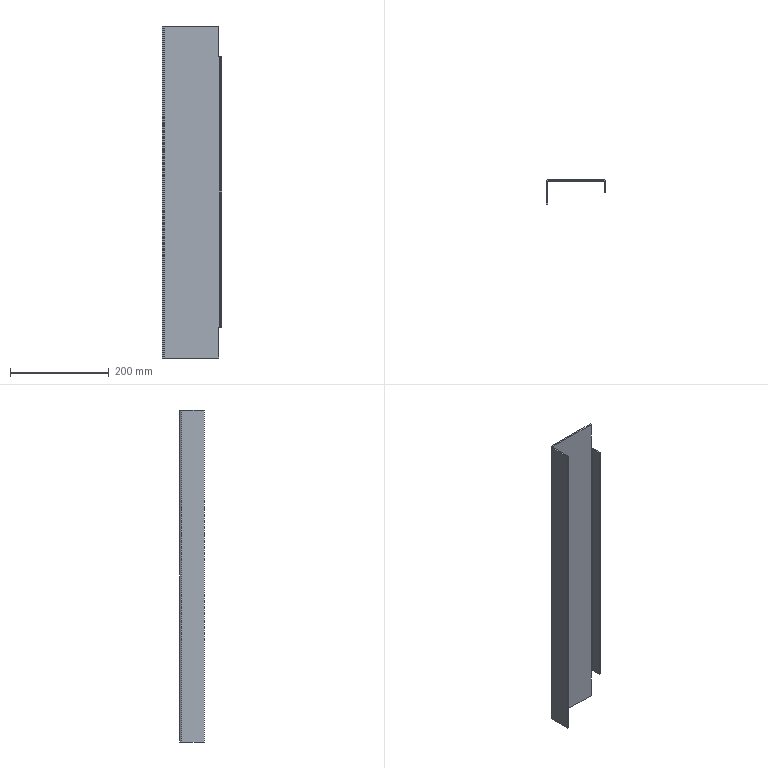Part | STEP file | 中转釜踏Plate 2 | 1 solid | 18 faces | box 120 x 50 x 674 mm | volume 367802 mm3 | plane 14 | cylinder 4 | commonest cylinder face diameters 2 x2 8 x2
STEP:
#1=CARTESIAN_POINT('',(0.,0.,0.));
#2=DIRECTION('',(0.,0.,1.));
#3=DIRECTION('',(1.,0.,0.));
#4=AXIS2_PLACEMENT_3D('',#1,#2,#3);
#5=CARTESIAN_POINT('',(-3.,-25.,275.));
#6=VERTEX_POINT('',#5);
#7=CARTESIAN_POINT('',(-3.,-25.,-275.));
#8=VERTEX_POINT('',#7);
#9=CARTESIAN_POINT('',(-3.,-25.,337.));
#10=DIRECTION('',(0.,0.,-1.));
#11=VECTOR('',#10,1.);
#12=LINE('',#9,#11);
#13=CARTESIAN_POINT('',(-3.,-4.,337.));
#14=DIRECTION('',(1.,0.,0.));
#15=DIRECTION('',(0.,1.,0.));
#16=AXIS2_PLACEMENT_3D('',#13,#14,#15);
#17=PLANE('',#16);
#18=CARTESIAN_POINT('',(-21.,0.));
#19=DIRECTION('',(0.,-1.));
#20=VECTOR('',#19,1.);
#21=LINE('',#18,#20);
#22=(GEOMETRIC_REPRESENTATION_CONTEXT(2)PARAMETRIC_REPRESENTATION_CONTEXT()REPRESENTATION_CONTEXT('',''));
#23=DEFINITIONAL_REPRESENTATION('',(#21),#22);
#24=PCURVE('',#17,#23);
#25=CARTESIAN_POINT('',(0.,-25.,337.));
#26=DIRECTION('',(0.,-1.,0.));
#27=DIRECTION('',(0.,0.,-1.));
#28=AXIS2_PLACEMENT_3D('',#25,#26,#27);
#29=PLANE('',#28);
#30=CARTESIAN_POINT('',(0.,-3.));
#31=DIRECTION('',(1.,0.));
#32=VECTOR('',#31,1.);
#33=LINE('',#30,#32);
#34=(GEOMETRIC_REPRESENTATION_CONTEXT(2)PARAMETRIC_REPRESENTATION_CONTEXT()REPRESENTATION_CONTEXT('',''));
#35=DEFINITIONAL_REPRESENTATION('',(#33),#34);
#36=PCURVE('',#29,#35);
#37=SURFACE_CURVE('',#12,(#24,#36),.PCURVE_S1.);
#38=EDGE_CURVE('',#6,#8,#37,.T.);
#39=ORIENTED_EDGE('',*,*,#38,.F.);
#40=CARTESIAN_POINT('',(-3.,-4.,275.));
#41=VERTEX_POINT('',#40);
#42=CARTESIAN_POINT('',(-3.,-4.,275.));
#43=DIRECTION('',(0.,1.,0.));
#44=VECTOR('',#43,1.);
#45=LINE('',#42,#44);
#46=CARTESIAN_POINT('',(0.,-62.));
#47=DIRECTION('',(1.,0.));
#48=VECTOR('',#47,1.);
#49=LINE('',#46,#48);
#50=(GEOMETRIC_REPRESENTATION_CONTEXT(2)PARAMETRIC_REPRESENTATION_CONTEXT()REPRESENTATION_CONTEXT('',''));
#51=DEFINITIONAL_REPRESENTATION('',(#49),#50);
#52=PCURVE('',#17,#51);
#53=CARTESIAN_POINT('',(0.,-50.,275.));
#54=DIRECTION('',(0.,0.,-1.));
#55=DIRECTION('',(-1.,0.,0.));
#56=AXIS2_PLACEMENT_3D('',#53,#54,#55);
#57=PLANE('',#56);
#58=CARTESIAN_POINT('',(3.,46.));
#59=DIRECTION('',(0.,1.));
#60=VECTOR('',#59,1.);
#61=LINE('',#58,#60);
#62=(GEOMETRIC_REPRESENTATION_CONTEXT(2)PARAMETRIC_REPRESENTATION_CONTEXT()REPRESENTATION_CONTEXT('',''));
#63=DEFINITIONAL_REPRESENTATION('',(#61),#62);
#64=PCURVE('',#57,#63);
#65=SURFACE_CURVE('',#45,(#52,#64),.PCURVE_S1.);
#66=EDGE_CURVE('',#6,#41,#65,.T.);
#67=ORIENTED_EDGE('',*,*,#66,.T.);
#68=CARTESIAN_POINT('',(-3.,-4.,-275.));
#69=VERTEX_POINT('',#68);
#70=CARTESIAN_POINT('',(-3.,-4.,337.));
#71=DIRECTION('',(0.,0.,-1.));
#72=VECTOR('',#71,1.);
#73=LINE('',#70,#72);
#74=CARTESIAN_POINT('',(0.,0.));
#75=DIRECTION('',(0.,-1.));
#76=VECTOR('',#75,1.);
#77=LINE('',#74,#76);
#78=(GEOMETRIC_REPRESENTATION_CONTEXT(2)PARAMETRIC_REPRESENTATION_CONTEXT()REPRESENTATION_CONTEXT('',''));
#79=DEFINITIONAL_REPRESENTATION('',(#77),#78);
#80=PCURVE('',#17,#79);
#81=CARTESIAN_POINT('',(-4.,-4.,337.));
#82=DIRECTION('',(0.,0.,-1.));
#83=DIRECTION('',(-1.,0.,0.));
#84=AXIS2_PLACEMENT_3D('',#81,#82,#83);
#85=CYLINDRICAL_SURFACE('',#84,1.);
#86=CARTESIAN_POINT('',(3.142,0.));
#87=DIRECTION('',(0.,1.));
#88=VECTOR('',#87,1.);
#89=LINE('',#86,#88);
#90=(GEOMETRIC_REPRESENTATION_CONTEXT(2)PARAMETRIC_REPRESENTATION_CONTEXT()REPRESENTATION_CONTEXT('',''));
#91=DEFINITIONAL_REPRESENTATION('',(#89),#90);
#92=PCURVE('',#85,#91);
#93=SURFACE_CURVE('',#73,(#80,#92),.PCURVE_S1.);
#94=EDGE_CURVE('',#41,#69,#93,.T.);
#95=ORIENTED_EDGE('',*,*,#94,.T.);
#96=CARTESIAN_POINT('',(-3.,-4.,-275.));
#97=DIRECTION('',(0.,-1.,0.));
#98=VECTOR('',#97,1.);
#99=LINE('',#96,#98);
#100=CARTESIAN_POINT('',(0.,-612.));
#101=DIRECTION('',(-1.,0.));
#102=VECTOR('',#101,1.);
#103=LINE('',#100,#102);
#104=(GEOMETRIC_REPRESENTATION_CONTEXT(2)PARAMETRIC_REPRESENTATION_CONTEXT()REPRESENTATION_CONTEXT('',''));
#105=DEFINITIONAL_REPRESENTATION('',(#103),#104);
#106=PCURVE('',#17,#105);
#107=CARTESIAN_POINT('',(0.,-50.,-275.));
#108=DIRECTION('',(0.,0.,1.));
#109=DIRECTION('',(1.,0.,0.));
#110=AXIS2_PLACEMENT_3D('',#107,#108,#109);
#111=PLANE('',#110);
#112=CARTESIAN_POINT('',(-3.,46.));
#113=DIRECTION('',(0.,-1.));
#114=VECTOR('',#113,1.);
#115=LINE('',#112,#114);
#116=(GEOMETRIC_REPRESENTATION_CONTEXT(2)PARAMETRIC_REPRESENTATION_CONTEXT()REPRESENTATION_CONTEXT('',''));
#117=DEFINITIONAL_REPRESENTATION('',(#115),#116);
#118=PCURVE('',#111,#117);
#119=SURFACE_CURVE('',#99,(#106,#118),.PCURVE_S1.);
#120=EDGE_CURVE('',#69,#8,#119,.T.);
#121=ORIENTED_EDGE('',*,*,#120,.T.);
#122=EDGE_LOOP('',(#39,#67,#95,#121));
#123=FACE_BOUND('',#122,.T.);
#124=ADVANCED_FACE('',(#123),#17,.F.);
#125=CARTESIAN_POINT('',(0.,-25.,275.));
#126=VERTEX_POINT('',#125);
#127=CARTESIAN_POINT('',(0.,-25.,275.));
#128=DIRECTION('',(1.,0.,0.));
#129=VECTOR('',#128,1.);
#130=LINE('',#127,#129);
#131=CARTESIAN_POINT('',(62.,0.));
#132=DIRECTION('',(0.,1.));
#133=VECTOR('',#132,1.);
#134=LINE('',#131,#133);
#135=(GEOMETRIC_REPRESENTATION_CONTEXT(2)PARAMETRIC_REPRESENTATION_CONTEXT()REPRESENTATION_CONTEXT('',''));
#136=DEFINITIONAL_REPRESENTATION('',(#134),#135);
#137=PCURVE('',#29,#136);
#138=CARTESIAN_POINT('',(0.,25.));
#139=DIRECTION('',(-1.,0.));
#140=VECTOR('',#139,1.);
#141=LINE('',#138,#140);
#142=(GEOMETRIC_REPRESENTATION_CONTEXT(2)PARAMETRIC_REPRESENTATION_CONTEXT()REPRESENTATION_CONTEXT('',''));
#143=DEFINITIONAL_REPRESENTATION('',(#141),#142);
#144=PCURVE('',#57,#143);
#145=SURFACE_CURVE('',#130,(#137,#144),.PCURVE_S1.);
#146=EDGE_CURVE('',#6,#126,#145,.T.);
#147=ORIENTED_EDGE('',*,*,#146,.F.);
#148=ORIENTED_EDGE('',*,*,#38,.T.);
#149=CARTESIAN_POINT('',(0.,-25.,-275.));
#150=VERTEX_POINT('',#149);
#151=CARTESIAN_POINT('',(0.,-25.,-275.));
#152=DIRECTION('',(-1.,0.,0.));
#153=VECTOR('',#152,1.);
#154=LINE('',#151,#153);
#155=CARTESIAN_POINT('',(612.,0.));
#156=DIRECTION('',(0.,-1.));
#157=VECTOR('',#156,1.);
#158=LINE('',#155,#157);
#159=(GEOMETRIC_REPRESENTATION_CONTEXT(2)PARAMETRIC_REPRESENTATION_CONTEXT()REPRESENTATION_CONTEXT('',''));
#160=DEFINITIONAL_REPRESENTATION('',(#158),#159);
#161=PCURVE('',#29,#160);
#162=CARTESIAN_POINT('',(0.,25.));
#163=DIRECTION('',(-1.,0.));
#164=VECTOR('',#163,1.);
#165=LINE('',#162,#164);
#166=(GEOMETRIC_REPRESENTATION_CONTEXT(2)PARAMETRIC_REPRESENTATION_CONTEXT()REPRESENTATION_CONTEXT('',''));
#167=DEFINITIONAL_REPRESENTATION('',(#165),#166);
#168=PCURVE('',#111,#167);
#169=SURFACE_CURVE('',#154,(#161,#168),.PCURVE_S1.);
#170=EDGE_CURVE('',#150,#8,#169,.T.);
#171=ORIENTED_EDGE('',*,*,#170,.F.);
#172=CARTESIAN_POINT('',(0.,-25.,337.));
#173=DIRECTION('',(0.,0.,-1.));
#174=VECTOR('',#173,1.);
#175=LINE('',#172,#174);
#176=CARTESIAN_POINT('',(0.,0.));
#177=DIRECTION('',(1.,0.));
#178=VECTOR('',#177,1.);
#179=LINE('',#176,#178);
#180=(GEOMETRIC_REPRESENTATION_CONTEXT(2)PARAMETRIC_REPRESENTATION_CONTEXT()REPRESENTATION_CONTEXT('',''));
#181=DEFINITIONAL_REPRESENTATION('',(#179),#180);
#182=PCURVE('',#29,#181);
#183=CARTESIAN_POINT('',(0.,-4.,337.));
#184=DIRECTION('',(1.,0.,0.));
#185=DIRECTION('',(0.,1.,0.));
#186=AXIS2_PLACEMENT_3D('',#183,#184,#185);
#187=PLANE('',#186);
#188=CARTESIAN_POINT('',(-21.,0.));
#189=DIRECTION('',(0.,-1.));
#190=VECTOR('',#189,1.);
#191=LINE('',#188,#190);
#192=(GEOMETRIC_REPRESENTATION_CONTEXT(2)PARAMETRIC_REPRESENTATION_CONTEXT()REPRESENTATION_CONTEXT('',''));
#193=DEFINITIONAL_REPRESENTATION('',(#191),#192);
#194=PCURVE('',#187,#193);
#195=SURFACE_CURVE('',#175,(#182,#194),.PCURVE_S1.);
#196=EDGE_CURVE('',#126,#150,#195,.T.);
#197=ORIENTED_EDGE('',*,*,#196,.F.);
#198=EDGE_LOOP('',(#147,#148,#171,#197));
#199=FACE_BOUND('',#198,.T.);
#200=ADVANCED_FACE('',(#199),#29,.T.);
#201=CARTESIAN_POINT('',(0.,-4.,275.));
#202=VERTEX_POINT('',#201);
#203=CARTESIAN_POINT('',(0.,-50.,275.));
#204=DIRECTION('',(0.,1.,0.));
#205=VECTOR('',#204,1.);
#206=LINE('',#203,#205);
#207=CARTESIAN_POINT('',(-46.,-62.));
#208=DIRECTION('',(1.,0.));
#209=VECTOR('',#208,1.);
#210=LINE('',#207,#209);
#211=(GEOMETRIC_REPRESENTATION_CONTEXT(2)PARAMETRIC_REPRESENTATION_CONTEXT()REPRESENTATION_CONTEXT('',''));
#212=DEFINITIONAL_REPRESENTATION('',(#210),#211);
#213=PCURVE('',#187,#212);
#214=CARTESIAN_POINT('',(0.,0.));
#215=DIRECTION('',(0.,1.));
#216=VECTOR('',#215,1.);
#217=LINE('',#214,#216);
#218=(GEOMETRIC_REPRESENTATION_CONTEXT(2)PARAMETRIC_REPRESENTATION_CONTEXT()REPRESENTATION_CONTEXT('',''));
#219=DEFINITIONAL_REPRESENTATION('',(#217),#218);
#220=PCURVE('',#57,#219);
#221=SURFACE_CURVE('',#206,(#213,#220),.PCURVE_S1.);
#222=EDGE_CURVE('',#126,#202,#221,.T.);
#223=ORIENTED_EDGE('',*,*,#222,.F.);
#224=ORIENTED_EDGE('',*,*,#196,.T.);
#225=CARTESIAN_POINT('',(0.,-4.,-275.));
#226=VERTEX_POINT('',#225);
#227=CARTESIAN_POINT('',(0.,-50.,-275.));
#228=DIRECTION('',(0.,1.,0.));
#229=VECTOR('',#228,1.);
#230=LINE('',#227,#229);
#231=CARTESIAN_POINT('',(-46.,-612.));
#232=DIRECTION('',(1.,0.));
#233=VECTOR('',#232,1.);
#234=LINE('',#231,#233);
#235=(GEOMETRIC_REPRESENTATION_CONTEXT(2)PARAMETRIC_REPRESENTATION_CONTEXT()REPRESENTATION_CONTEXT('',''));
#236=DEFINITIONAL_REPRESENTATION('',(#234),#235);
#237=PCURVE('',#187,#236);
#238=CARTESIAN_POINT('',(0.,0.));
#239=DIRECTION('',(0.,1.));
#240=VECTOR('',#239,1.);
#241=LINE('',#238,#240);
#242=(GEOMETRIC_REPRESENTATION_CONTEXT(2)PARAMETRIC_REPRESENTATION_CONTEXT()REPRESENTATION_CONTEXT('',''));
#243=DEFINITIONAL_REPRESENTATION('',(#241),#242);
#244=PCURVE('',#111,#243);
#245=SURFACE_CURVE('',#230,(#237,#244),.PCURVE_S1.);
#246=EDGE_CURVE('',#150,#226,#245,.T.);
#247=ORIENTED_EDGE('',*,*,#246,.T.);
#248=CARTESIAN_POINT('',(0.,-4.,337.));
#249=DIRECTION('',(0.,0.,-1.));
#250=VECTOR('',#249,1.);
#251=LINE('',#248,#250);
#252=CARTESIAN_POINT('',(0.,0.));
#253=DIRECTION('',(0.,-1.));
#254=VECTOR('',#253,1.);
#255=LINE('',#252,#254);
#256=(GEOMETRIC_REPRESENTATION_CONTEXT(2)PARAMETRIC_REPRESENTATION_CONTEXT()REPRESENTATION_CONTEXT('',''));
#257=DEFINITIONAL_REPRESENTATION('',(#255),#256);
#258=PCURVE('',#187,#257);
#259=CARTESIAN_POINT('',(-4.,-4.,337.));
#260=DIRECTION('',(0.,0.,-1.));
#261=DIRECTION('',(-1.,0.,0.));
#262=AXIS2_PLACEMENT_3D('',#259,#260,#261);
#263=CYLINDRICAL_SURFACE('',#262,4.);
#264=CARTESIAN_POINT('',(3.142,0.));
#265=DIRECTION('',(0.,1.));
#266=VECTOR('',#265,1.);
#267=LINE('',#264,#266);
#268=(GEOMETRIC_REPRESENTATION_CONTEXT(2)PARAMETRIC_REPRESENTATION_CONTEXT()REPRESENTATION_CONTEXT('',''));
#269=DEFINITIONAL_REPRESENTATION('',(#267),#268);
#270=PCURVE('',#263,#269);
#271=SURFACE_CURVE('',#251,(#258,#270),.PCURVE_S1.);
#272=EDGE_CURVE('',#202,#226,#271,.T.);
#273=ORIENTED_EDGE('',*,*,#272,.F.);
#274=EDGE_LOOP('',(#223,#224,#247,#273));
#275=FACE_BOUND('',#274,.T.);
#276=ADVANCED_FACE('',(#275),#187,.T.);
#277=CARTESIAN_POINT('',(-4.,0.,275.));
#278=VERTEX_POINT('',#277);
#279=CARTESIAN_POINT('',(-4.,-4.,275.));
#280=DIRECTION('',(0.,0.,1.));
#281=DIRECTION('',(-1.,0.,0.));
#282=AXIS2_PLACEMENT_3D('',#279,#280,#281);
#283=CIRCLE('',#282,4.);
#284=CARTESIAN_POINT('',(6.283,62.));
#285=DIRECTION('',(-1.,0.));
#286=VECTOR('',#285,1.);
#287=LINE('',#284,#286);
#288=(GEOMETRIC_REPRESENTATION_CONTEXT(2)PARAMETRIC_REPRESENTATION_CONTEXT()REPRESENTATION_CONTEXT('',''));
#289=DEFINITIONAL_REPRESENTATION('',(#287),#288);
#290=PCURVE('',#263,#289);
#291=CARTESIAN_POINT('',(8.,46.));
#292=CARTESIAN_POINT('',(8.,39.072));
#293=CARTESIAN_POINT('',(2.,42.536));
#294=CARTESIAN_POINT('',(-4.,46.));
#295=CARTESIAN_POINT('',(2.,49.464));
#296=CARTESIAN_POINT('',(8.,52.928));
#297=CARTESIAN_POINT('',(8.,46.));
#298=(BOUNDED_CURVE()B_SPLINE_CURVE(2,(#291,#292,#293,#294,#295,#296,#297),.UNSPECIFIED.,.T.,.F.)B_SPLINE_CURVE_WITH_KNOTS((1,2,2,2,2,1),(-2.094,0.,2.094,4.189,6.283,8.378),.UNSPECIFIED.)CURVE()GEOMETRIC_REPRESENTATION_ITEM()RATIONAL_B_SPLINE_CURVE((1.,0.5,1.,0.5,1.,0.5,1.))REPRESENTATION_ITEM(''));
#299=(GEOMETRIC_REPRESENTATION_CONTEXT(2)PARAMETRIC_REPRESENTATION_CONTEXT()REPRESENTATION_CONTEXT('',''));
#300=DEFINITIONAL_REPRESENTATION('',(#298),#299);
#301=PCURVE('',#57,#300);
#302=SURFACE_CURVE('',#283,(#290,#301),.PCURVE_S1.);
#303=EDGE_CURVE('',#202,#278,#302,.T.);
#304=ORIENTED_EDGE('',*,*,#303,.F.);
#305=ORIENTED_EDGE('',*,*,#272,.T.);
#306=CARTESIAN_POINT('',(-4.,0.,-275.));
#307=VERTEX_POINT('',#306);
#308=CARTESIAN_POINT('',(-4.,-4.,-275.));
#309=DIRECTION('',(0.,0.,-1.));
#310=DIRECTION('',(1.,0.,0.));
#311=AXIS2_PLACEMENT_3D('',#308,#309,#310);
#312=CIRCLE('',#311,4.);
#313=CARTESIAN_POINT('',(-3.142,612.));
#314=DIRECTION('',(1.,0.));
#315=VECTOR('',#314,1.);
#316=LINE('',#313,#315);
#317=(GEOMETRIC_REPRESENTATION_CONTEXT(2)PARAMETRIC_REPRESENTATION_CONTEXT()REPRESENTATION_CONTEXT('',''));
#318=DEFINITIONAL_REPRESENTATION('',(#316),#317);
#319=PCURVE('',#263,#318);
#320=CARTESIAN_POINT('',(0.,46.));
#321=CARTESIAN_POINT('',(0.,39.072));
#322=CARTESIAN_POINT('',(-6.,42.536));
#323=CARTESIAN_POINT('',(-12.,46.));
#324=CARTESIAN_POINT('',(-6.,49.464));
#325=CARTESIAN_POINT('',(0.,52.928));
#326=CARTESIAN_POINT('',(0.,46.));
#327=(BOUNDED_CURVE()B_SPLINE_CURVE(2,(#320,#321,#322,#323,#324,#325,#326),.UNSPECIFIED.,.T.,.F.)B_SPLINE_CURVE_WITH_KNOTS((1,2,2,2,2,1),(-2.094,0.,2.094,4.189,6.283,8.378),.UNSPECIFIED.)CURVE()GEOMETRIC_REPRESENTATION_ITEM()RATIONAL_B_SPLINE_CURVE((1.,0.5,1.,0.5,1.,0.5,1.))REPRESENTATION_ITEM(''));
#328=(GEOMETRIC_REPRESENTATION_CONTEXT(2)PARAMETRIC_REPRESENTATION_CONTEXT()REPRESENTATION_CONTEXT('',''));
#329=DEFINITIONAL_REPRESENTATION('',(#327),#328);
#330=PCURVE('',#111,#329);
#331=SURFACE_CURVE('',#312,(#319,#330),.PCURVE_S1.);
#332=EDGE_CURVE('',#307,#226,#331,.T.);
#333=ORIENTED_EDGE('',*,*,#332,.F.);
#334=CARTESIAN_POINT('',(-4.,0.,337.));
#335=DIRECTION('',(0.,0.,-1.));
#336=VECTOR('',#335,1.);
#337=LINE('',#334,#336);
#338=CARTESIAN_POINT('',(1.571,0.));
#339=DIRECTION('',(0.,1.));
#340=VECTOR('',#339,1.);
#341=LINE('',#338,#340);
#342=(GEOMETRIC_REPRESENTATION_CONTEXT(2)PARAMETRIC_REPRESENTATION_CONTEXT()REPRESENTATION_CONTEXT('',''));
#343=DEFINITIONAL_REPRESENTATION('',(#341),#342);
#344=PCURVE('',#263,#343);
#345=CARTESIAN_POINT('',(-116.,0.,337.));
#346=DIRECTION('',(0.,1.,0.));
#347=DIRECTION('',(0.,0.,1.));
#348=AXIS2_PLACEMENT_3D('',#345,#346,#347);
#349=PLANE('',#348);
#350=CARTESIAN_POINT('',(0.,112.));
#351=DIRECTION('',(-1.,0.));
#352=VECTOR('',#351,1.);
#353=LINE('',#350,#352);
#354=(GEOMETRIC_REPRESENTATION_CONTEXT(2)PARAMETRIC_REPRESENTATION_CONTEXT()REPRESENTATION_CONTEXT('',''));
#355=DEFINITIONAL_REPRESENTATION('',(#353),#354);
#356=PCURVE('',#349,#355);
#357=SURFACE_CURVE('',#337,(#344,#356),.PCURVE_S1.);
#358=EDGE_CURVE('',#278,#307,#357,.T.);
#359=ORIENTED_EDGE('',*,*,#358,.F.);
#360=EDGE_LOOP('',(#304,#305,#333,#359));
#361=FACE_BOUND('',#360,.T.);
#362=ADVANCED_FACE('',(#361),#263,.T.);
#363=CARTESIAN_POINT('',(-6.,0.,275.));
#364=VERTEX_POINT('',#363);
#365=CARTESIAN_POINT('',(-6.,0.,337.));
#366=VERTEX_POINT('',#365);
#367=CARTESIAN_POINT('',(-6.,0.,337.));
#368=DIRECTION('',(0.,0.,1.));
#369=VECTOR('',#368,1.);
#370=LINE('',#367,#369);
#371=CARTESIAN_POINT('',(0.,110.));
#372=DIRECTION('',(1.,0.));
#373=VECTOR('',#372,1.);
#374=LINE('',#371,#373);
#375=(GEOMETRIC_REPRESENTATION_CONTEXT(2)PARAMETRIC_REPRESENTATION_CONTEXT()REPRESENTATION_CONTEXT('',''));
#376=DEFINITIONAL_REPRESENTATION('',(#374),#375);
#377=PCURVE('',#349,#376);
#378=CARTESIAN_POINT('',(-6.,-50.,337.));
#379=DIRECTION('',(-1.,0.,0.));
#380=DIRECTION('',(0.,0.,1.));
#381=AXIS2_PLACEMENT_3D('',#378,#379,#380);
#382=PLANE('',#381);
#383=CARTESIAN_POINT('',(0.,50.));
#384=DIRECTION('',(1.,0.));
#385=VECTOR('',#384,1.);
#386=LINE('',#383,#385);
#387=(GEOMETRIC_REPRESENTATION_CONTEXT(2)PARAMETRIC_REPRESENTATION_CONTEXT()REPRESENTATION_CONTEXT('',''));
#388=DEFINITIONAL_REPRESENTATION('',(#386),#387);
#389=PCURVE('',#382,#388);
#390=SURFACE_CURVE('',#370,(#377,#389),.PCURVE_S1.);
#391=EDGE_CURVE('',#364,#366,#390,.T.);
#392=ORIENTED_EDGE('',*,*,#391,.F.);
#393=CARTESIAN_POINT('',(-116.,0.,275.));
#394=DIRECTION('',(-1.,0.,0.));
#395=VECTOR('',#394,1.);
#396=LINE('',#393,#395);
#397=CARTESIAN_POINT('',(-62.,0.));
#398=DIRECTION('',(0.,-1.));
#399=VECTOR('',#398,1.);
#400=LINE('',#397,#399);
#401=(GEOMETRIC_REPRESENTATION_CONTEXT(2)PARAMETRIC_REPRESENTATION_CONTEXT()REPRESENTATION_CONTEXT('',''));
#402=DEFINITIONAL_REPRESENTATION('',(#400),#401);
#403=PCURVE('',#349,#402);
#404=CARTESIAN_POINT('',(116.,50.));
#405=DIRECTION('',(1.,0.));
#406=VECTOR('',#405,1.);
#407=LINE('',#404,#406);
#408=(GEOMETRIC_REPRESENTATION_CONTEXT(2)PARAMETRIC_REPRESENTATION_CONTEXT()REPRESENTATION_CONTEXT('',''));
#409=DEFINITIONAL_REPRESENTATION('',(#407),#408);
#410=PCURVE('',#57,#409);
#411=SURFACE_CURVE('',#396,(#403,#410),.PCURVE_S1.);
#412=EDGE_CURVE('',#278,#364,#411,.T.);
#413=ORIENTED_EDGE('',*,*,#412,.F.);
#414=ORIENTED_EDGE('',*,*,#358,.T.);
#415=CARTESIAN_POINT('',(-6.,0.,-275.));
#416=VERTEX_POINT('',#415);
#417=CARTESIAN_POINT('',(-116.,0.,-275.));
#418=DIRECTION('',(1.,0.,0.));
#419=VECTOR('',#418,1.);
#420=LINE('',#417,#419);
#421=CARTESIAN_POINT('',(-612.,0.));
#422=DIRECTION('',(0.,1.));
#423=VECTOR('',#422,1.);
#424=LINE('',#421,#423);
#425=(GEOMETRIC_REPRESENTATION_CONTEXT(2)PARAMETRIC_REPRESENTATION_CONTEXT()REPRESENTATION_CONTEXT('',''));
#426=DEFINITIONAL_REPRESENTATION('',(#424),#425);
#427=PCURVE('',#349,#426);
#428=CARTESIAN_POINT('',(-116.,50.));
#429=DIRECTION('',(1.,0.));
#430=VECTOR('',#429,1.);
#431=LINE('',#428,#430);
#432=(GEOMETRIC_REPRESENTATION_CONTEXT(2)PARAMETRIC_REPRESENTATION_CONTEXT()REPRESENTATION_CONTEXT('',''));
#433=DEFINITIONAL_REPRESENTATION('',(#431),#432);
#434=PCURVE('',#111,#433);
#435=SURFACE_CURVE('',#420,(#427,#434),.PCURVE_S1.);
#436=EDGE_CURVE('',#416,#307,#435,.T.);
#437=ORIENTED_EDGE('',*,*,#436,.F.);
#438=CARTESIAN_POINT('',(-6.,0.,-337.));
#439=VERTEX_POINT('',#438);
#440=CARTESIAN_POINT('',(-6.,0.,337.));
#441=DIRECTION('',(0.,0.,1.));
#442=VECTOR('',#441,1.);
#443=LINE('',#440,#442);
#444=CARTESIAN_POINT('',(0.,110.));
#445=DIRECTION('',(1.,0.));
#446=VECTOR('',#445,1.);
#447=LINE('',#444,#446);
#448=(GEOMETRIC_REPRESENTATION_CONTEXT(2)PARAMETRIC_REPRESENTATION_CONTEXT()REPRESENTATION_CONTEXT('',''));
#449=DEFINITIONAL_REPRESENTATION('',(#447),#448);
#450=PCURVE('',#349,#449);
#451=CARTESIAN_POINT('',(-6.,-50.,-337.));
#452=DIRECTION('',(-1.,0.,0.));
#453=DIRECTION('',(0.,0.,1.));
#454=AXIS2_PLACEMENT_3D('',#451,#452,#453);
#455=PLANE('',#454);
#456=CARTESIAN_POINT('',(674.,50.));
#457=DIRECTION('',(1.,0.));
#458=VECTOR('',#457,1.);
#459=LINE('',#456,#458);
#460=(GEOMETRIC_REPRESENTATION_CONTEXT(2)PARAMETRIC_REPRESENTATION_CONTEXT()REPRESENTATION_CONTEXT('',''));
#461=DEFINITIONAL_REPRESENTATION('',(#459),#460);
#462=PCURVE('',#455,#461);
#463=SURFACE_CURVE('',#443,(#450,#462),.PCURVE_S1.);
#464=EDGE_CURVE('',#439,#416,#463,.T.);
#465=ORIENTED_EDGE('',*,*,#464,.F.);
#466=CARTESIAN_POINT('',(-116.,0.,-337.));
#467=VERTEX_POINT('',#466);
#468=CARTESIAN_POINT('',(-116.,0.,-337.));
#469=DIRECTION('',(1.,0.,0.));
#470=VECTOR('',#469,1.);
#471=LINE('',#468,#470);
#472=CARTESIAN_POINT('',(-674.,0.));
#473=DIRECTION('',(0.,1.));
#474=VECTOR('',#473,1.);
#475=LINE('',#472,#474);
#476=(GEOMETRIC_REPRESENTATION_CONTEXT(2)PARAMETRIC_REPRESENTATION_CONTEXT()REPRESENTATION_CONTEXT('',''));
#477=DEFINITIONAL_REPRESENTATION('',(#475),#476);
#478=PCURVE('',#349,#477);
#479=CARTESIAN_POINT('',(-4.,-4.,-337.));
#480=DIRECTION('',(0.,0.,-1.));
#481=DIRECTION('',(-1.,0.,0.));
#482=AXIS2_PLACEMENT_3D('',#479,#480,#481);
#483=PLANE('',#482);
#484=CARTESIAN_POINT('',(112.,4.));
#485=DIRECTION('',(-1.,0.));
#486=VECTOR('',#485,1.);
#487=LINE('',#484,#486);
#488=(GEOMETRIC_REPRESENTATION_CONTEXT(2)PARAMETRIC_REPRESENTATION_CONTEXT()REPRESENTATION_CONTEXT('',''));
#489=DEFINITIONAL_REPRESENTATION('',(#487),#488);
#490=PCURVE('',#483,#489);
#491=SURFACE_CURVE('',#471,(#478,#490),.PCURVE_S1.);
#492=EDGE_CURVE('',#467,#439,#491,.T.);
#493=ORIENTED_EDGE('',*,*,#492,.F.);
#494=CARTESIAN_POINT('',(-116.,0.,337.));
#495=VERTEX_POINT('',#494);
#496=CARTESIAN_POINT('',(-116.,0.,337.));
#497=DIRECTION('',(0.,0.,-1.));
#498=VECTOR('',#497,1.);
#499=LINE('',#496,#498);
#500=CARTESIAN_POINT('',(0.,0.));
#501=DIRECTION('',(-1.,0.));
#502=VECTOR('',#501,1.);
#503=LINE('',#500,#502);
#504=(GEOMETRIC_REPRESENTATION_CONTEXT(2)PARAMETRIC_REPRESENTATION_CONTEXT()REPRESENTATION_CONTEXT('',''));
#505=DEFINITIONAL_REPRESENTATION('',(#503),#504);
#506=PCURVE('',#349,#505);
#507=CARTESIAN_POINT('',(-116.,-4.,337.));
#508=DIRECTION('',(0.,0.,-1.));
#509=DIRECTION('',(-1.,0.,0.));
#510=AXIS2_PLACEMENT_3D('',#507,#508,#509);
#511=CYLINDRICAL_SURFACE('',#510,4.);
#512=CARTESIAN_POINT('',(1.571,0.));
#513=DIRECTION('',(0.,1.));
#514=VECTOR('',#513,1.);
#515=LINE('',#512,#514);
#516=(GEOMETRIC_REPRESENTATION_CONTEXT(2)PARAMETRIC_REPRESENTATION_CONTEXT()REPRESENTATION_CONTEXT('',''));
#517=DEFINITIONAL_REPRESENTATION('',(#515),#516);
#518=PCURVE('',#511,#517);
#519=SURFACE_CURVE('',#499,(#506,#518),.PCURVE_S1.);
#520=EDGE_CURVE('',#495,#467,#519,.T.);
#521=ORIENTED_EDGE('',*,*,#520,.F.);
#522=CARTESIAN_POINT('',(-116.,0.,337.));
#523=DIRECTION('',(1.,0.,0.));
#524=VECTOR('',#523,1.);
#525=LINE('',#522,#524);
#526=CARTESIAN_POINT('',(0.,0.));
#527=DIRECTION('',(0.,1.));
#528=VECTOR('',#527,1.);
#529=LINE('',#526,#528);
#530=(GEOMETRIC_REPRESENTATION_CONTEXT(2)PARAMETRIC_REPRESENTATION_CONTEXT()REPRESENTATION_CONTEXT('',''));
#531=DEFINITIONAL_REPRESENTATION('',(#529),#530);
#532=PCURVE('',#349,#531);
#533=CARTESIAN_POINT('',(-4.,-4.,337.));
#534=DIRECTION('',(0.,0.,-1.));
#535=DIRECTION('',(-1.,0.,0.));
#536=AXIS2_PLACEMENT_3D('',#533,#534,#535);
#537=PLANE('',#536);
#538=CARTESIAN_POINT('',(112.,4.));
#539=DIRECTION('',(-1.,0.));
#540=VECTOR('',#539,1.);
#541=LINE('',#538,#540);
#542=(GEOMETRIC_REPRESENTATION_CONTEXT(2)PARAMETRIC_REPRESENTATION_CONTEXT()REPRESENTATION_CONTEXT('',''));
#543=DEFINITIONAL_REPRESENTATION('',(#541),#542);
#544=PCURVE('',#537,#543);
#545=SURFACE_CURVE('',#525,(#532,#544),.PCURVE_S1.);
#546=EDGE_CURVE('',#495,#366,#545,.T.);
#547=ORIENTED_EDGE('',*,*,#546,.T.);
#548=EDGE_LOOP('',(#392,#413,#414,#437,#465,#493,#521,#547));
#549=FACE_BOUND('',#548,.T.);
#550=ADVANCED_FACE('',(#549),#349,.T.);
#551=CARTESIAN_POINT('',(-120.,-4.,-337.));
#552=VERTEX_POINT('',#551);
#553=CARTESIAN_POINT('',(-116.,-4.,-337.));
#554=DIRECTION('',(0.,0.,-1.));
#555=DIRECTION('',(1.,0.,0.));
#556=AXIS2_PLACEMENT_3D('',#553,#554,#555);
#557=CIRCLE('',#556,4.);
#558=CARTESIAN_POINT('',(-3.142,674.));
#559=DIRECTION('',(1.,0.));
#560=VECTOR('',#559,1.);
#561=LINE('',#558,#560);
#562=(GEOMETRIC_REPRESENTATION_CONTEXT(2)PARAMETRIC_REPRESENTATION_CONTEXT()REPRESENTATION_CONTEXT('',''));
#563=DEFINITIONAL_REPRESENTATION('',(#561),#562);
#564=PCURVE('',#511,#563);
#565=CARTESIAN_POINT('',(112.,0.));
#566=DIRECTION('',(-1.,0.));
#567=AXIS2_PLACEMENT_2D('',#565,#566);
#568=CIRCLE('',#567,4.);
#569=(GEOMETRIC_REPRESENTATION_CONTEXT(2)PARAMETRIC_REPRESENTATION_CONTEXT()REPRESENTATION_CONTEXT('',''));
#570=DEFINITIONAL_REPRESENTATION('',(#568),#569);
#571=PCURVE('',#483,#570);
#572=SURFACE_CURVE('',#557,(#564,#571),.PCURVE_S1.);
#573=EDGE_CURVE('',#552,#467,#572,.T.);
#574=ORIENTED_EDGE('',*,*,#573,.F.);
#575=CARTESIAN_POINT('',(-120.,-4.,337.));
#576=VERTEX_POINT('',#575);
#577=CARTESIAN_POINT('',(-120.,-4.,337.));
#578=DIRECTION('',(0.,0.,-1.));
#579=VECTOR('',#578,1.);
#580=LINE('',#577,#579);
#581=CARTESIAN_POINT('',(0.,0.));
#582=DIRECTION('',(0.,1.));
#583=VECTOR('',#582,1.);
#584=LINE('',#581,#583);
#585=(GEOMETRIC_REPRESENTATION_CONTEXT(2)PARAMETRIC_REPRESENTATION_CONTEXT()REPRESENTATION_CONTEXT('',''));
#586=DEFINITIONAL_REPRESENTATION('',(#584),#585);
#587=PCURVE('',#511,#586);
#588=CARTESIAN_POINT('',(-120.,-4.,337.));
#589=DIRECTION('',(-1.,0.,0.));
#590=DIRECTION('',(0.,0.,1.));
#591=AXIS2_PLACEMENT_3D('',#588,#589,#590);
#592=PLANE('',#591);
#593=CARTESIAN_POINT('',(0.,0.));
#594=DIRECTION('',(-1.,0.));
#595=VECTOR('',#594,1.);
#596=LINE('',#593,#595);
#597=(GEOMETRIC_REPRESENTATION_CONTEXT(2)PARAMETRIC_REPRESENTATION_CONTEXT()REPRESENTATION_CONTEXT('',''));
#598=DEFINITIONAL_REPRESENTATION('',(#596),#597);
#599=PCURVE('',#592,#598);
#600=SURFACE_CURVE('',#580,(#587,#599),.PCURVE_S1.);
#601=EDGE_CURVE('',#576,#552,#600,.T.);
#602=ORIENTED_EDGE('',*,*,#601,.F.);
#603=CARTESIAN_POINT('',(-116.,-4.,337.));
#604=DIRECTION('',(0.,0.,-1.));
#605=DIRECTION('',(1.,0.,0.));
#606=AXIS2_PLACEMENT_3D('',#603,#604,#605);
#607=CIRCLE('',#606,4.);
#608=CARTESIAN_POINT('',(-3.142,0.));
#609=DIRECTION('',(1.,0.));
#610=VECTOR('',#609,1.);
#611=LINE('',#608,#610);
#612=(GEOMETRIC_REPRESENTATION_CONTEXT(2)PARAMETRIC_REPRESENTATION_CONTEXT()REPRESENTATION_CONTEXT('',''));
#613=DEFINITIONAL_REPRESENTATION('',(#611),#612);
#614=PCURVE('',#511,#613);
#615=CARTESIAN_POINT('',(112.,0.));
#616=DIRECTION('',(-1.,0.));
#617=AXIS2_PLACEMENT_2D('',#615,#616);
#618=CIRCLE('',#617,4.);
#619=(GEOMETRIC_REPRESENTATION_CONTEXT(2)PARAMETRIC_REPRESENTATION_CONTEXT()REPRESENTATION_CONTEXT('',''));
#620=DEFINITIONAL_REPRESENTATION('',(#618),#619);
#621=PCURVE('',#537,#620);
#622=SURFACE_CURVE('',#607,(#614,#621),.PCURVE_S1.);
#623=EDGE_CURVE('',#576,#495,#622,.T.);
#624=ORIENTED_EDGE('',*,*,#623,.T.);
#625=ORIENTED_EDGE('',*,*,#520,.T.);
#626=EDGE_LOOP('',(#574,#602,#624,#625));
#627=FACE_BOUND('',#626,.T.);
#628=ADVANCED_FACE('',(#627),#511,.T.);
#629=CARTESIAN_POINT('',(-120.,-50.,-337.));
#630=VERTEX_POINT('',#629);
#631=CARTESIAN_POINT('',(-120.,-4.,-337.));
#632=DIRECTION('',(0.,1.,0.));
#633=VECTOR('',#632,1.);
#634=LINE('',#631,#633);
#635=CARTESIAN_POINT('',(-674.,0.));
#636=DIRECTION('',(0.,1.));
#637=VECTOR('',#636,1.);
#638=LINE('',#635,#637);
#639=(GEOMETRIC_REPRESENTATION_CONTEXT(2)PARAMETRIC_REPRESENTATION_CONTEXT()REPRESENTATION_CONTEXT('',''));
#640=DEFINITIONAL_REPRESENTATION('',(#638),#639);
#641=PCURVE('',#592,#640);
#642=CARTESIAN_POINT('',(116.,0.));
#643=DIRECTION('',(0.,1.));
#644=VECTOR('',#643,1.);
#645=LINE('',#642,#644);
#646=(GEOMETRIC_REPRESENTATION_CONTEXT(2)PARAMETRIC_REPRESENTATION_CONTEXT()REPRESENTATION_CONTEXT('',''));
#647=DEFINITIONAL_REPRESENTATION('',(#645),#646);
#648=PCURVE('',#483,#647);
#649=SURFACE_CURVE('',#634,(#641,#648),.PCURVE_S1.);
#650=EDGE_CURVE('',#630,#552,#649,.T.);
#651=ORIENTED_EDGE('',*,*,#650,.F.);
#652=CARTESIAN_POINT('',(-120.,-50.,337.));
#653=VERTEX_POINT('',#652);
#654=CARTESIAN_POINT('',(-120.,-50.,337.));
#655=DIRECTION('',(0.,0.,-1.));
#656=VECTOR('',#655,1.);
#657=LINE('',#654,#656);
#658=CARTESIAN_POINT('',(0.,-46.));
#659=DIRECTION('',(-1.,0.));
#660=VECTOR('',#659,1.);
#661=LINE('',#658,#660);
#662=(GEOMETRIC_REPRESENTATION_CONTEXT(2)PARAMETRIC_REPRESENTATION_CONTEXT()REPRESENTATION_CONTEXT('',''));
#663=DEFINITIONAL_REPRESENTATION('',(#661),#662);
#664=PCURVE('',#592,#663);
#665=CARTESIAN_POINT('',(-117.,-50.,337.));
#666=DIRECTION('',(0.,-1.,0.));
#667=DIRECTION('',(0.,0.,-1.));
#668=AXIS2_PLACEMENT_3D('',#665,#666,#667);
#669=PLANE('',#668);
#670=CARTESIAN_POINT('',(0.,-3.));
#671=DIRECTION('',(1.,0.));
#672=VECTOR('',#671,1.);
#673=LINE('',#670,#672);
#674=(GEOMETRIC_REPRESENTATION_CONTEXT(2)PARAMETRIC_REPRESENTATION_CONTEXT()REPRESENTATION_CONTEXT('',''));
#675=DEFINITIONAL_REPRESENTATION('',(#673),#674);
#676=PCURVE('',#669,#675);
#677=SURFACE_CURVE('',#657,(#664,#676),.PCURVE_S1.);
#678=EDGE_CURVE('',#653,#630,#677,.T.);
#679=ORIENTED_EDGE('',*,*,#678,.F.);
#680=CARTESIAN_POINT('',(-120.,-4.,337.));
#681=DIRECTION('',(0.,1.,0.));
#682=VECTOR('',#681,1.);
#683=LINE('',#680,#682);
#684=CARTESIAN_POINT('',(0.,0.));
#685=DIRECTION('',(0.,1.));
#686=VECTOR('',#685,1.);
#687=LINE('',#684,#686);
#688=(GEOMETRIC_REPRESENTATION_CONTEXT(2)PARAMETRIC_REPRESENTATION_CONTEXT()REPRESENTATION_CONTEXT('',''));
#689=DEFINITIONAL_REPRESENTATION('',(#687),#688);
#690=PCURVE('',#592,#689);
#691=CARTESIAN_POINT('',(116.,0.));
#692=DIRECTION('',(0.,1.));
#693=VECTOR('',#692,1.);
#694=LINE('',#691,#693);
#695=(GEOMETRIC_REPRESENTATION_CONTEXT(2)PARAMETRIC_REPRESENTATION_CONTEXT()REPRESENTATION_CONTEXT('',''));
#696=DEFINITIONAL_REPRESENTATION('',(#694),#695);
#697=PCURVE('',#537,#696);
#698=SURFACE_CURVE('',#683,(#690,#697),.PCURVE_S1.);
#699=EDGE_CURVE('',#653,#576,#698,.T.);
#700=ORIENTED_EDGE('',*,*,#699,.T.);
#701=ORIENTED_EDGE('',*,*,#601,.T.);
#702=EDGE_LOOP('',(#651,#679,#700,#701));
#703=FACE_BOUND('',#702,.T.);
#704=ADVANCED_FACE('',(#703),#592,.T.);
#705=CARTESIAN_POINT('',(-117.,-50.,-337.));
#706=VERTEX_POINT('',#705);
#707=CARTESIAN_POINT('',(-117.,-50.,-337.));
#708=DIRECTION('',(-1.,0.,0.));
#709=VECTOR('',#708,1.);
#710=LINE('',#707,#709);
#711=CARTESIAN_POINT('',(674.,0.));
#712=DIRECTION('',(0.,-1.));
#713=VECTOR('',#712,1.);
#714=LINE('',#711,#713);
#715=(GEOMETRIC_REPRESENTATION_CONTEXT(2)PARAMETRIC_REPRESENTATION_CONTEXT()REPRESENTATION_CONTEXT('',''));
#716=DEFINITIONAL_REPRESENTATION('',(#714),#715);
#717=PCURVE('',#669,#716);
#718=CARTESIAN_POINT('',(113.,-46.));
#719=DIRECTION('',(1.,0.));
#720=VECTOR('',#719,1.);
#721=LINE('',#718,#720);
#722=(GEOMETRIC_REPRESENTATION_CONTEXT(2)PARAMETRIC_REPRESENTATION_CONTEXT()REPRESENTATION_CONTEXT('',''));
#723=DEFINITIONAL_REPRESENTATION('',(#721),#722);
#724=PCURVE('',#483,#723);
#725=SURFACE_CURVE('',#710,(#717,#724),.PCURVE_S1.);
#726=EDGE_CURVE('',#706,#630,#725,.T.);
#727=ORIENTED_EDGE('',*,*,#726,.F.);
#728=CARTESIAN_POINT('',(-117.,-50.,337.));
#729=VERTEX_POINT('',#728);
#730=CARTESIAN_POINT('',(-117.,-50.,337.));
#731=DIRECTION('',(0.,0.,-1.));
#732=VECTOR('',#731,1.);
#733=LINE('',#730,#732);
#734=CARTESIAN_POINT('',(0.,0.));
#735=DIRECTION('',(1.,0.));
#736=VECTOR('',#735,1.);
#737=LINE('',#734,#736);
#738=(GEOMETRIC_REPRESENTATION_CONTEXT(2)PARAMETRIC_REPRESENTATION_CONTEXT()REPRESENTATION_CONTEXT('',''));
#739=DEFINITIONAL_REPRESENTATION('',(#737),#738);
#740=PCURVE('',#669,#739);
#741=CARTESIAN_POINT('',(-117.,-4.,337.));
#742=DIRECTION('',(-1.,0.,0.));
#743=DIRECTION('',(0.,0.,1.));
#744=AXIS2_PLACEMENT_3D('',#741,#742,#743);
#745=PLANE('',#744);
#746=CARTESIAN_POINT('',(0.,-46.));
#747=DIRECTION('',(-1.,0.));
#748=VECTOR('',#747,1.);
#749=LINE('',#746,#748);
#750=(GEOMETRIC_REPRESENTATION_CONTEXT(2)PARAMETRIC_REPRESENTATION_CONTEXT()REPRESENTATION_CONTEXT('',''));
#751=DEFINITIONAL_REPRESENTATION('',(#749),#750);
#752=PCURVE('',#745,#751);
#753=SURFACE_CURVE('',#733,(#740,#752),.PCURVE_S1.);
#754=EDGE_CURVE('',#729,#706,#753,.T.);
#755=ORIENTED_EDGE('',*,*,#754,.F.);
#756=CARTESIAN_POINT('',(-117.,-50.,337.));
#757=DIRECTION('',(-1.,0.,0.));
#758=VECTOR('',#757,1.);
#759=LINE('',#756,#758);
#760=CARTESIAN_POINT('',(0.,0.));
#761=DIRECTION('',(0.,-1.));
#762=VECTOR('',#761,1.);
#763=LINE('',#760,#762);
#764=(GEOMETRIC_REPRESENTATION_CONTEXT(2)PARAMETRIC_REPRESENTATION_CONTEXT()REPRESENTATION_CONTEXT('',''));
#765=DEFINITIONAL_REPRESENTATION('',(#763),#764);
#766=PCURVE('',#669,#765);
#767=CARTESIAN_POINT('',(113.,-46.));
#768=DIRECTION('',(1.,0.));
#769=VECTOR('',#768,1.);
#770=LINE('',#767,#769);
#771=(GEOMETRIC_REPRESENTATION_CONTEXT(2)PARAMETRIC_REPRESENTATION_CONTEXT()REPRESENTATION_CONTEXT('',''));
#772=DEFINITIONAL_REPRESENTATION('',(#770),#771);
#773=PCURVE('',#537,#772);
#774=SURFACE_CURVE('',#759,(#766,#773),.PCURVE_S1.);
#775=EDGE_CURVE('',#729,#653,#774,.T.);
#776=ORIENTED_EDGE('',*,*,#775,.T.);
#777=ORIENTED_EDGE('',*,*,#678,.T.);
#778=EDGE_LOOP('',(#727,#755,#776,#777));
#779=FACE_BOUND('',#778,.T.);
#780=ADVANCED_FACE('',(#779),#669,.T.);
#781=CARTESIAN_POINT('',(-117.,-4.,-337.));
#782=VERTEX_POINT('',#781);
#783=CARTESIAN_POINT('',(-117.,-4.,-337.));
#784=DIRECTION('',(0.,1.,0.));
#785=VECTOR('',#784,1.);
#786=LINE('',#783,#785);
#787=CARTESIAN_POINT('',(-674.,0.));
#788=DIRECTION('',(0.,1.));
#789=VECTOR('',#788,1.);
#790=LINE('',#787,#789);
#791=(GEOMETRIC_REPRESENTATION_CONTEXT(2)PARAMETRIC_REPRESENTATION_CONTEXT()REPRESENTATION_CONTEXT('',''));
#792=DEFINITIONAL_REPRESENTATION('',(#790),#791);
#793=PCURVE('',#745,#792);
#794=CARTESIAN_POINT('',(113.,0.));
#795=DIRECTION('',(0.,1.));
#796=VECTOR('',#795,1.);
#797=LINE('',#794,#796);
#798=(GEOMETRIC_REPRESENTATION_CONTEXT(2)PARAMETRIC_REPRESENTATION_CONTEXT()REPRESENTATION_CONTEXT('',''));
#799=DEFINITIONAL_REPRESENTATION('',(#797),#798);
#800=PCURVE('',#483,#799);
#801=SURFACE_CURVE('',#786,(#793,#800),.PCURVE_S1.);
#802=EDGE_CURVE('',#706,#782,#801,.T.);
#803=ORIENTED_EDGE('',*,*,#802,.T.);
#804=CARTESIAN_POINT('',(-117.,-4.,337.));
#805=VERTEX_POINT('',#804);
#806=CARTESIAN_POINT('',(-117.,-4.,337.));
#807=DIRECTION('',(0.,0.,-1.));
#808=VECTOR('',#807,1.);
#809=LINE('',#806,#808);
#810=CARTESIAN_POINT('',(0.,0.));
#811=DIRECTION('',(-1.,0.));
#812=VECTOR('',#811,1.);
#813=LINE('',#810,#812);
#814=(GEOMETRIC_REPRESENTATION_CONTEXT(2)PARAMETRIC_REPRESENTATION_CONTEXT()REPRESENTATION_CONTEXT('',''));
#815=DEFINITIONAL_REPRESENTATION('',(#813),#814);
#816=PCURVE('',#745,#815);
#817=CARTESIAN_POINT('',(-116.,-4.,337.));
#818=DIRECTION('',(0.,0.,-1.));
#819=DIRECTION('',(-1.,0.,0.));
#820=AXIS2_PLACEMENT_3D('',#817,#818,#819);
#821=CYLINDRICAL_SURFACE('',#820,1.);
#822=CARTESIAN_POINT('',(0.,0.));
#823=DIRECTION('',(0.,1.));
#824=VECTOR('',#823,1.);
#825=LINE('',#822,#824);
#826=(GEOMETRIC_REPRESENTATION_CONTEXT(2)PARAMETRIC_REPRESENTATION_CONTEXT()REPRESENTATION_CONTEXT('',''));
#827=DEFINITIONAL_REPRESENTATION('',(#825),#826);
#828=PCURVE('',#821,#827);
#829=SURFACE_CURVE('',#809,(#816,#828),.PCURVE_S1.);
#830=EDGE_CURVE('',#805,#782,#829,.T.);
#831=ORIENTED_EDGE('',*,*,#830,.F.);
#832=CARTESIAN_POINT('',(-117.,-4.,337.));
#833=DIRECTION('',(0.,1.,0.));
#834=VECTOR('',#833,1.);
#835=LINE('',#832,#834);
#836=CARTESIAN_POINT('',(0.,0.));
#837=DIRECTION('',(0.,1.));
#838=VECTOR('',#837,1.);
#839=LINE('',#836,#838);
#840=(GEOMETRIC_REPRESENTATION_CONTEXT(2)PARAMETRIC_REPRESENTATION_CONTEXT()REPRESENTATION_CONTEXT('',''));
#841=DEFINITIONAL_REPRESENTATION('',(#839),#840);
#842=PCURVE('',#745,#841);
#843=CARTESIAN_POINT('',(113.,0.));
#844=DIRECTION('',(0.,1.));
#845=VECTOR('',#844,1.);
#846=LINE('',#843,#845);
#847=(GEOMETRIC_REPRESENTATION_CONTEXT(2)PARAMETRIC_REPRESENTATION_CONTEXT()REPRESENTATION_CONTEXT('',''));
#848=DEFINITIONAL_REPRESENTATION('',(#846),#847);
#849=PCURVE('',#537,#848);
#850=SURFACE_CURVE('',#835,(#842,#849),.PCURVE_S1.);
#851=EDGE_CURVE('',#729,#805,#850,.T.);
#852=ORIENTED_EDGE('',*,*,#851,.F.);
#853=ORIENTED_EDGE('',*,*,#754,.T.);
#854=EDGE_LOOP('',(#803,#831,#852,#853));
#855=FACE_BOUND('',#854,.T.);
#856=ADVANCED_FACE('',(#855),#745,.F.);
#857=ORIENTED_EDGE('',*,*,#830,.F.);
#858=CARTESIAN_POINT('',(-116.,-3.,337.));
#859=VERTEX_POINT('',#858);
#860=CARTESIAN_POINT('',(-116.,-4.,337.));
#861=DIRECTION('',(0.,0.,-1.));
#862=DIRECTION('',(1.,0.,0.));
#863=AXIS2_PLACEMENT_3D('',#860,#861,#862);
#864=CIRCLE('',#863,1.);
#865=CARTESIAN_POINT('',(-3.142,0.));
#866=DIRECTION('',(1.,0.));
#867=VECTOR('',#866,1.);
#868=LINE('',#865,#867);
#869=(GEOMETRIC_REPRESENTATION_CONTEXT(2)PARAMETRIC_REPRESENTATION_CONTEXT()REPRESENTATION_CONTEXT('',''));
#870=DEFINITIONAL_REPRESENTATION('',(#868),#869);
#871=PCURVE('',#821,#870);
#872=CARTESIAN_POINT('',(112.,0.));
#873=DIRECTION('',(-1.,0.));
#874=AXIS2_PLACEMENT_2D('',#872,#873);
#875=CIRCLE('',#874,1.);
#876=(GEOMETRIC_REPRESENTATION_CONTEXT(2)PARAMETRIC_REPRESENTATION_CONTEXT()REPRESENTATION_CONTEXT('',''));
#877=DEFINITIONAL_REPRESENTATION('',(#875),#876);
#878=PCURVE('',#537,#877);
#879=SURFACE_CURVE('',#864,(#871,#878),.PCURVE_S1.);
#880=EDGE_CURVE('',#805,#859,#879,.T.);
#881=ORIENTED_EDGE('',*,*,#880,.T.);
#882=CARTESIAN_POINT('',(-116.,-3.,-337.));
#883=VERTEX_POINT('',#882);
#884=CARTESIAN_POINT('',(-116.,-3.,337.));
#885=DIRECTION('',(0.,0.,-1.));
#886=VECTOR('',#885,1.);
#887=LINE('',#884,#886);
#888=CARTESIAN_POINT('',(1.571,0.));
#889=DIRECTION('',(0.,1.));
#890=VECTOR('',#889,1.);
#891=LINE('',#888,#890);
#892=(GEOMETRIC_REPRESENTATION_CONTEXT(2)PARAMETRIC_REPRESENTATION_CONTEXT()REPRESENTATION_CONTEXT('',''));
#893=DEFINITIONAL_REPRESENTATION('',(#891),#892);
#894=PCURVE('',#821,#893);
#895=CARTESIAN_POINT('',(-116.,-3.,337.));
#896=DIRECTION('',(0.,1.,0.));
#897=DIRECTION('',(0.,0.,1.));
#898=AXIS2_PLACEMENT_3D('',#895,#896,#897);
#899=PLANE('',#898);
#900=CARTESIAN_POINT('',(0.,0.));
#901=DIRECTION('',(-1.,0.));
#902=VECTOR('',#901,1.);
#903=LINE('',#900,#902);
#904=(GEOMETRIC_REPRESENTATION_CONTEXT(2)PARAMETRIC_REPRESENTATION_CONTEXT()REPRESENTATION_CONTEXT('',''));
#905=DEFINITIONAL_REPRESENTATION('',(#903),#904);
#906=PCURVE('',#899,#905);
#907=SURFACE_CURVE('',#887,(#894,#906),.PCURVE_S1.);
#908=EDGE_CURVE('',#859,#883,#907,.T.);
#909=ORIENTED_EDGE('',*,*,#908,.T.);
#910=CARTESIAN_POINT('',(-116.,-4.,-337.));
#911=DIRECTION('',(0.,0.,-1.));
#912=DIRECTION('',(1.,0.,0.));
#913=AXIS2_PLACEMENT_3D('',#910,#911,#912);
#914=CIRCLE('',#913,1.);
#915=CARTESIAN_POINT('',(-3.142,674.));
#916=DIRECTION('',(1.,0.));
#917=VECTOR('',#916,1.);
#918=LINE('',#915,#917);
#919=(GEOMETRIC_REPRESENTATION_CONTEXT(2)PARAMETRIC_REPRESENTATION_CONTEXT()REPRESENTATION_CONTEXT('',''));
#920=DEFINITIONAL_REPRESENTATION('',(#918),#919);
#921=PCURVE('',#821,#920);
#922=CARTESIAN_POINT('',(112.,0.));
#923=DIRECTION('',(-1.,0.));
#924=AXIS2_PLACEMENT_2D('',#922,#923);
#925=CIRCLE('',#924,1.);
#926=(GEOMETRIC_REPRESENTATION_CONTEXT(2)PARAMETRIC_REPRESENTATION_CONTEXT()REPRESENTATION_CONTEXT('',''));
#927=DEFINITIONAL_REPRESENTATION('',(#925),#926);
#928=PCURVE('',#483,#927);
#929=SURFACE_CURVE('',#914,(#921,#928),.PCURVE_S1.);
#930=EDGE_CURVE('',#782,#883,#929,.T.);
#931=ORIENTED_EDGE('',*,*,#930,.F.);
#932=EDGE_LOOP('',(#857,#881,#909,#931));
#933=FACE_BOUND('',#932,.F.);
#934=ADVANCED_FACE('',(#933),#821,.F.);
#935=CARTESIAN_POINT('',(-4.,-3.,275.));
#936=VERTEX_POINT('',#935);
#937=CARTESIAN_POINT('',(-6.,-3.,275.));
#938=VERTEX_POINT('',#937);
#939=CARTESIAN_POINT('',(-116.,-3.,275.));
#940=DIRECTION('',(-1.,0.,0.));
#941=VECTOR('',#940,1.);
#942=LINE('',#939,#941);
#943=CARTESIAN_POINT('',(-62.,0.));
#944=DIRECTION('',(0.,-1.));
#945=VECTOR('',#944,1.);
#946=LINE('',#943,#945);
#947=(GEOMETRIC_REPRESENTATION_CONTEXT(2)PARAMETRIC_REPRESENTATION_CONTEXT()REPRESENTATION_CONTEXT('',''));
#948=DEFINITIONAL_REPRESENTATION('',(#946),#947);
#949=PCURVE('',#899,#948);
#950=CARTESIAN_POINT('',(116.,47.));
#951=DIRECTION('',(1.,0.));
#952=VECTOR('',#951,1.);
#953=LINE('',#950,#952);
#954=(GEOMETRIC_REPRESENTATION_CONTEXT(2)PARAMETRIC_REPRESENTATION_CONTEXT()REPRESENTATION_CONTEXT('',''));
#955=DEFINITIONAL_REPRESENTATION('',(#953),#954);
#956=PCURVE('',#57,#955);
#957=SURFACE_CURVE('',#942,(#949,#956),.PCURVE_S1.);
#958=EDGE_CURVE('',#936,#938,#957,.T.);
#959=ORIENTED_EDGE('',*,*,#958,.T.);
#960=CARTESIAN_POINT('',(-6.,-3.,337.));
#961=VERTEX_POINT('',#960);
#962=CARTESIAN_POINT('',(-6.,-3.,337.));
#963=DIRECTION('',(0.,0.,1.));
#964=VECTOR('',#963,1.);
#965=LINE('',#962,#964);
#966=CARTESIAN_POINT('',(0.,110.));
#967=DIRECTION('',(1.,0.));
#968=VECTOR('',#967,1.);
#969=LINE('',#966,#968);
#970=(GEOMETRIC_REPRESENTATION_CONTEXT(2)PARAMETRIC_REPRESENTATION_CONTEXT()REPRESENTATION_CONTEXT('',''));
#971=DEFINITIONAL_REPRESENTATION('',(#969),#970);
#972=PCURVE('',#899,#971);
#973=CARTESIAN_POINT('',(0.,47.));
#974=DIRECTION('',(1.,0.));
#975=VECTOR('',#974,1.);
#976=LINE('',#973,#975);
#977=(GEOMETRIC_REPRESENTATION_CONTEXT(2)PARAMETRIC_REPRESENTATION_CONTEXT()REPRESENTATION_CONTEXT('',''));
#978=DEFINITIONAL_REPRESENTATION('',(#976),#977);
#979=PCURVE('',#382,#978);
#980=SURFACE_CURVE('',#965,(#972,#979),.PCURVE_S1.);
#981=EDGE_CURVE('',#938,#961,#980,.T.);
#982=ORIENTED_EDGE('',*,*,#981,.T.);
#983=CARTESIAN_POINT('',(-116.,-3.,337.));
#984=DIRECTION('',(1.,0.,0.));
#985=VECTOR('',#984,1.);
#986=LINE('',#983,#985);
#987=CARTESIAN_POINT('',(0.,0.));
#988=DIRECTION('',(0.,1.));
#989=VECTOR('',#988,1.);
#990=LINE('',#987,#989);
#991=(GEOMETRIC_REPRESENTATION_CONTEXT(2)PARAMETRIC_REPRESENTATION_CONTEXT()REPRESENTATION_CONTEXT('',''));
#992=DEFINITIONAL_REPRESENTATION('',(#990),#991);
#993=PCURVE('',#899,#992);
#994=CARTESIAN_POINT('',(112.,1.));
#995=DIRECTION('',(-1.,0.));
#996=VECTOR('',#995,1.);
#997=LINE('',#994,#996);
#998=(GEOMETRIC_REPRESENTATION_CONTEXT(2)PARAMETRIC_REPRESENTATION_CONTEXT()REPRESENTATION_CONTEXT('',''));
#999=DEFINITIONAL_REPRESENTATION('',(#997),#998);
#1000=PCURVE('',#537,#999);
#1001=SURFACE_CURVE('',#986,(#993,#1000),.PCURVE_S1.);
#1002=EDGE_CURVE('',#859,#961,#1001,.T.);
#1003=ORIENTED_EDGE('',*,*,#1002,.F.);
#1004=ORIENTED_EDGE('',*,*,#908,.T.);
#1005=CARTESIAN_POINT('',(-6.,-3.,-337.));
#1006=VERTEX_POINT('',#1005);
#1007=CARTESIAN_POINT('',(-116.,-3.,-337.));
#1008=DIRECTION('',(1.,0.,0.));
#1009=VECTOR('',#1008,1.);
#1010=LINE('',#1007,#1009);
#1011=CARTESIAN_POINT('',(-674.,0.));
#1012=DIRECTION('',(0.,1.));
#1013=VECTOR('',#1012,1.);
#1014=LINE('',#1011,#1013);
#1015=(GEOMETRIC_REPRESENTATION_CONTEXT(2)PARAMETRIC_REPRESENTATION_CONTEXT()REPRESENTATION_CONTEXT('',''));
#1016=DEFINITIONAL_REPRESENTATION('',(#1014),#1015);
#1017=PCURVE('',#899,#1016);
#1018=CARTESIAN_POINT('',(112.,1.));
#1019=DIRECTION('',(-1.,0.));
#1020=VECTOR('',#1019,1.);
#1021=LINE('',#1018,#1020);
#1022=(GEOMETRIC_REPRESENTATION_CONTEXT(2)PARAMETRIC_REPRESENTATION_CONTEXT()REPRESENTATION_CONTEXT('',''));
#1023=DEFINITIONAL_REPRESENTATION('',(#1021),#1022);
#1024=PCURVE('',#483,#1023);
#1025=SURFACE_CURVE('',#1010,(#1017,#1024),.PCURVE_S1.);
#1026=EDGE_CURVE('',#883,#1006,#1025,.T.);
#1027=ORIENTED_EDGE('',*,*,#1026,.T.);
#1028=CARTESIAN_POINT('',(-6.,-3.,-275.));
#1029=VERTEX_POINT('',#1028);
#1030=CARTESIAN_POINT('',(-6.,-3.,337.));
#1031=DIRECTION('',(0.,0.,1.));
#1032=VECTOR('',#1031,1.);
#1033=LINE('',#1030,#1032);
#1034=CARTESIAN_POINT('',(0.,110.));
#1035=DIRECTION('',(1.,0.));
#1036=VECTOR('',#1035,1.);
#1037=LINE('',#1034,#1036);
#1038=(GEOMETRIC_REPRESENTATION_CONTEXT(2)PARAMETRIC_REPRESENTATION_CONTEXT()REPRESENTATION_CONTEXT('',''));
#1039=DEFINITIONAL_REPRESENTATION('',(#1037),#1038);
#1040=PCURVE('',#899,#1039);
#1041=CARTESIAN_POINT('',(674.,47.));
#1042=DIRECTION('',(1.,0.));
#1043=VECTOR('',#1042,1.);
#1044=LINE('',#1041,#1043);
#1045=(GEOMETRIC_REPRESENTATION_CONTEXT(2)PARAMETRIC_REPRESENTATION_CONTEXT()REPRESENTATION_CONTEXT('',''));
#1046=DEFINITIONAL_REPRESENTATION('',(#1044),#1045);
#1047=PCURVE('',#455,#1046);
#1048=SURFACE_CURVE('',#1033,(#1040,#1047),.PCURVE_S1.);
#1049=EDGE_CURVE('',#1006,#1029,#1048,.T.);
#1050=ORIENTED_EDGE('',*,*,#1049,.T.);
#1051=CARTESIAN_POINT('',(-4.,-3.,-275.));
#1052=VERTEX_POINT('',#1051);
#1053=CARTESIAN_POINT('',(-116.,-3.,-275.));
#1054=DIRECTION('',(1.,0.,0.));
#1055=VECTOR('',#1054,1.);
#1056=LINE('',#1053,#1055);
#1057=CARTESIAN_POINT('',(-612.,0.));
#1058=DIRECTION('',(0.,1.));
#1059=VECTOR('',#1058,1.);
#1060=LINE('',#1057,#1059);
#1061=(GEOMETRIC_REPRESENTATION_CONTEXT(2)PARAMETRIC_REPRESENTATION_CONTEXT()REPRESENTATION_CONTEXT('',''));
#1062=DEFINITIONAL_REPRESENTATION('',(#1060),#1061);
#1063=PCURVE('',#899,#1062);
#1064=CARTESIAN_POINT('',(-116.,47.));
#1065=DIRECTION('',(1.,0.));
#1066=VECTOR('',#1065,1.);
#1067=LINE('',#1064,#1066);
#1068=(GEOMETRIC_REPRESENTATION_CONTEXT(2)PARAMETRIC_REPRESENTATION_CONTEXT()REPRESENTATION_CONTEXT('',''));
#1069=DEFINITIONAL_REPRESENTATION('',(#1067),#1068);
#1070=PCURVE('',#111,#1069);
#1071=SURFACE_CURVE('',#1056,(#1063,#1070),.PCURVE_S1.);
#1072=EDGE_CURVE('',#1029,#1052,#1071,.T.);
#1073=ORIENTED_EDGE('',*,*,#1072,.T.);
#1074=CARTESIAN_POINT('',(-4.,-3.,337.));
#1075=DIRECTION('',(0.,0.,-1.));
#1076=VECTOR('',#1075,1.);
#1077=LINE('',#1074,#1076);
#1078=CARTESIAN_POINT('',(0.,112.));
#1079=DIRECTION('',(-1.,0.));
#1080=VECTOR('',#1079,1.);
#1081=LINE('',#1078,#1080);
#1082=(GEOMETRIC_REPRESENTATION_CONTEXT(2)PARAMETRIC_REPRESENTATION_CONTEXT()REPRESENTATION_CONTEXT('',''));
#1083=DEFINITIONAL_REPRESENTATION('',(#1081),#1082);
#1084=PCURVE('',#899,#1083);
#1085=CARTESIAN_POINT('',(1.571,0.));
#1086=DIRECTION('',(0.,1.));
#1087=VECTOR('',#1086,1.);
#1088=LINE('',#1085,#1087);
#1089=(GEOMETRIC_REPRESENTATION_CONTEXT(2)PARAMETRIC_REPRESENTATION_CONTEXT()REPRESENTATION_CONTEXT('',''));
#1090=DEFINITIONAL_REPRESENTATION('',(#1088),#1089);
#1091=PCURVE('',#85,#1090);
#1092=SURFACE_CURVE('',#1077,(#1084,#1091),.PCURVE_S1.);
#1093=EDGE_CURVE('',#936,#1052,#1092,.T.);
#1094=ORIENTED_EDGE('',*,*,#1093,.F.);
#1095=EDGE_LOOP('',(#959,#982,#1003,#1004,#1027,#1050,#1073,#1094));
#1096=FACE_BOUND('',#1095,.T.);
#1097=ADVANCED_FACE('',(#1096),#899,.F.);
#1098=CARTESIAN_POINT('',(-4.,-4.,-275.));
#1099=DIRECTION('',(0.,0.,-1.));
#1100=DIRECTION('',(1.,0.,0.));
#1101=AXIS2_PLACEMENT_3D('',#1098,#1099,#1100);
#1102=CIRCLE('',#1101,1.);
#1103=CARTESIAN_POINT('',(-3.142,612.));
#1104=DIRECTION('',(1.,0.));
#1105=VECTOR('',#1104,1.);
#1106=LINE('',#1103,#1105);
#1107=(GEOMETRIC_REPRESENTATION_CONTEXT(2)PARAMETRIC_REPRESENTATION_CONTEXT()REPRESENTATION_CONTEXT('',''));
#1108=DEFINITIONAL_REPRESENTATION('',(#1106),#1107);
#1109=PCURVE('',#85,#1108);
#1110=CARTESIAN_POINT('',(-3.,46.));
#1111=CARTESIAN_POINT('',(-3.,44.268));
#1112=CARTESIAN_POINT('',(-4.5,45.134));
#1113=CARTESIAN_POINT('',(-6.,46.));
#1114=CARTESIAN_POINT('',(-4.5,46.866));
#1115=CARTESIAN_POINT('',(-3.,47.732));
#1116=CARTESIAN_POINT('',(-3.,46.));
#1117=(BOUNDED_CURVE()B_SPLINE_CURVE(2,(#1110,#1111,#1112,#1113,#1114,#1115,#1116),.UNSPECIFIED.,.T.,.F.)B_SPLINE_CURVE_WITH_KNOTS((1,2,2,2,2,1),(-2.094,0.,2.094,4.189,6.283,8.378),.UNSPECIFIED.)CURVE()GEOMETRIC_REPRESENTATION_ITEM()RATIONAL_B_SPLINE_CURVE((1.,0.5,1.,0.5,1.,0.5,1.))REPRESENTATION_ITEM(''));
#1118=(GEOMETRIC_REPRESENTATION_CONTEXT(2)PARAMETRIC_REPRESENTATION_CONTEXT()REPRESENTATION_CONTEXT('',''));
#1119=DEFINITIONAL_REPRESENTATION('',(#1117),#1118);
#1120=PCURVE('',#111,#1119);
#1121=SURFACE_CURVE('',#1102,(#1109,#1120),.PCURVE_S1.);
#1122=EDGE_CURVE('',#1052,#69,#1121,.T.);
#1123=ORIENTED_EDGE('',*,*,#1122,.F.);
#1124=ORIENTED_EDGE('',*,*,#1093,.F.);
#1125=CARTESIAN_POINT('',(-4.,-4.,275.));
#1126=DIRECTION('',(0.,0.,1.));
#1127=DIRECTION('',(-1.,0.,0.));
#1128=AXIS2_PLACEMENT_3D('',#1125,#1126,#1127);
#1129=CIRCLE('',#1128,1.);
#1130=CARTESIAN_POINT('',(6.283,62.));
#1131=DIRECTION('',(-1.,0.));
#1132=VECTOR('',#1131,1.);
#1133=LINE('',#1130,#1132);
#1134=(GEOMETRIC_REPRESENTATION_CONTEXT(2)PARAMETRIC_REPRESENTATION_CONTEXT()REPRESENTATION_CONTEXT('',''));
#1135=DEFINITIONAL_REPRESENTATION('',(#1133),#1134);
#1136=PCURVE('',#85,#1135);
#1137=CARTESIAN_POINT('',(5.,46.));
#1138=CARTESIAN_POINT('',(5.,44.268));
#1139=CARTESIAN_POINT('',(3.5,45.134));
#1140=CARTESIAN_POINT('',(2.,46.));
#1141=CARTESIAN_POINT('',(3.5,46.866));
#1142=CARTESIAN_POINT('',(5.,47.732));
#1143=CARTESIAN_POINT('',(5.,46.));
#1144=(BOUNDED_CURVE()B_SPLINE_CURVE(2,(#1137,#1138,#1139,#1140,#1141,#1142,#1143),.UNSPECIFIED.,.T.,.F.)B_SPLINE_CURVE_WITH_KNOTS((1,2,2,2,2,1),(-2.094,0.,2.094,4.189,6.283,8.378),.UNSPECIFIED.)CURVE()GEOMETRIC_REPRESENTATION_ITEM()RATIONAL_B_SPLINE_CURVE((1.,0.5,1.,0.5,1.,0.5,1.))REPRESENTATION_ITEM(''));
#1145=(GEOMETRIC_REPRESENTATION_CONTEXT(2)PARAMETRIC_REPRESENTATION_CONTEXT()REPRESENTATION_CONTEXT('',''));
#1146=DEFINITIONAL_REPRESENTATION('',(#1144),#1145);
#1147=PCURVE('',#57,#1146);
#1148=SURFACE_CURVE('',#1129,(#1136,#1147),.PCURVE_S1.);
#1149=EDGE_CURVE('',#41,#936,#1148,.T.);
#1150=ORIENTED_EDGE('',*,*,#1149,.F.);
#1151=ORIENTED_EDGE('',*,*,#94,.T.);
#1152=EDGE_LOOP('',(#1123,#1124,#1150,#1151));
#1153=FACE_BOUND('',#1152,.F.);
#1154=ADVANCED_FACE('',(#1153),#85,.F.);
#1155=ORIENTED_EDGE('',*,*,#1002,.T.);
#1156=CARTESIAN_POINT('',(-6.,-4.,337.));
#1157=DIRECTION('',(0.,1.,0.));
#1158=VECTOR('',#1157,1.);
#1159=LINE('',#1156,#1158);
#1160=CARTESIAN_POINT('',(2.,0.));
#1161=DIRECTION('',(0.,1.));
#1162=VECTOR('',#1161,1.);
#1163=LINE('',#1160,#1162);
#1164=(GEOMETRIC_REPRESENTATION_CONTEXT(2)PARAMETRIC_REPRESENTATION_CONTEXT()REPRESENTATION_CONTEXT('',''));
#1165=DEFINITIONAL_REPRESENTATION('',(#1163),#1164);
#1166=PCURVE('',#537,#1165);
#1167=CARTESIAN_POINT('',(0.,46.));
#1168=DIRECTION('',(0.,1.));
#1169=VECTOR('',#1168,1.);
#1170=LINE('',#1167,#1169);
#1171=(GEOMETRIC_REPRESENTATION_CONTEXT(2)PARAMETRIC_REPRESENTATION_CONTEXT()REPRESENTATION_CONTEXT('',''));
#1172=DEFINITIONAL_REPRESENTATION('',(#1170),#1171);
#1173=PCURVE('',#382,#1172);
#1174=SURFACE_CURVE('',#1159,(#1166,#1173),.PCURVE_S1.);
#1175=EDGE_CURVE('',#961,#366,#1174,.T.);
#1176=ORIENTED_EDGE('',*,*,#1175,.T.);
#1177=ORIENTED_EDGE('',*,*,#546,.F.);
#1178=ORIENTED_EDGE('',*,*,#623,.F.);
#1179=ORIENTED_EDGE('',*,*,#699,.F.);
#1180=ORIENTED_EDGE('',*,*,#775,.F.);
#1181=ORIENTED_EDGE('',*,*,#851,.T.);
#1182=ORIENTED_EDGE('',*,*,#880,.T.);
#1183=EDGE_LOOP('',(#1155,#1176,#1177,#1178,#1179,#1180,#1181,#1182));
#1184=FACE_BOUND('',#1183,.T.);
#1185=ADVANCED_FACE('',(#1184),#537,.F.);
#1186=CARTESIAN_POINT('',(-6.,-4.,-337.));
#1187=DIRECTION('',(0.,1.,0.));
#1188=VECTOR('',#1187,1.);
#1189=LINE('',#1186,#1188);
#1190=CARTESIAN_POINT('',(2.,0.));
#1191=DIRECTION('',(0.,1.));
#1192=VECTOR('',#1191,1.);
#1193=LINE('',#1190,#1192);
#1194=(GEOMETRIC_REPRESENTATION_CONTEXT(2)PARAMETRIC_REPRESENTATION_CONTEXT()REPRESENTATION_CONTEXT('',''));
#1195=DEFINITIONAL_REPRESENTATION('',(#1193),#1194);
#1196=PCURVE('',#483,#1195);
#1197=CARTESIAN_POINT('',(0.,46.));
#1198=DIRECTION('',(0.,1.));
#1199=VECTOR('',#1198,1.);
#1200=LINE('',#1197,#1199);
#1201=(GEOMETRIC_REPRESENTATION_CONTEXT(2)PARAMETRIC_REPRESENTATION_CONTEXT()REPRESENTATION_CONTEXT('',''));
#1202=DEFINITIONAL_REPRESENTATION('',(#1200),#1201);
#1203=PCURVE('',#455,#1202);
#1204=SURFACE_CURVE('',#1189,(#1196,#1203),.PCURVE_S1.);
#1205=EDGE_CURVE('',#1006,#439,#1204,.T.);
#1206=ORIENTED_EDGE('',*,*,#1205,.F.);
#1207=ORIENTED_EDGE('',*,*,#1026,.F.);
#1208=ORIENTED_EDGE('',*,*,#930,.F.);
#1209=ORIENTED_EDGE('',*,*,#802,.F.);
#1210=ORIENTED_EDGE('',*,*,#726,.T.);
#1211=ORIENTED_EDGE('',*,*,#650,.T.);
#1212=ORIENTED_EDGE('',*,*,#573,.T.);
#1213=ORIENTED_EDGE('',*,*,#492,.T.);
#1214=EDGE_LOOP('',(#1206,#1207,#1208,#1209,#1210,#1211,#1212,#1213));
#1215=FACE_BOUND('',#1214,.T.);
#1216=ADVANCED_FACE('',(#1215),#483,.T.);
#1217=ORIENTED_EDGE('',*,*,#464,.T.);
#1218=CARTESIAN_POINT('',(-6.,-50.,-275.));
#1219=DIRECTION('',(0.,1.,0.));
#1220=VECTOR('',#1219,1.);
#1221=LINE('',#1218,#1220);
#1222=CARTESIAN_POINT('',(62.,0.));
#1223=DIRECTION('',(0.,1.));
#1224=VECTOR('',#1223,1.);
#1225=LINE('',#1222,#1224);
#1226=(GEOMETRIC_REPRESENTATION_CONTEXT(2)PARAMETRIC_REPRESENTATION_CONTEXT()REPRESENTATION_CONTEXT('',''));
#1227=DEFINITIONAL_REPRESENTATION('',(#1225),#1226);
#1228=PCURVE('',#455,#1227);
#1229=CARTESIAN_POINT('',(-6.,0.));
#1230=DIRECTION('',(0.,1.));
#1231=VECTOR('',#1230,1.);
#1232=LINE('',#1229,#1231);
#1233=(GEOMETRIC_REPRESENTATION_CONTEXT(2)PARAMETRIC_REPRESENTATION_CONTEXT()REPRESENTATION_CONTEXT('',''));
#1234=DEFINITIONAL_REPRESENTATION('',(#1232),#1233);
#1235=PCURVE('',#111,#1234);
#1236=SURFACE_CURVE('',#1221,(#1228,#1235),.PCURVE_S1.);
#1237=EDGE_CURVE('',#1029,#416,#1236,.T.);
#1238=ORIENTED_EDGE('',*,*,#1237,.F.);
#1239=ORIENTED_EDGE('',*,*,#1049,.F.);
#1240=ORIENTED_EDGE('',*,*,#1205,.T.);
#1241=EDGE_LOOP('',(#1217,#1238,#1239,#1240));
#1242=FACE_BOUND('',#1241,.T.);
#1243=ADVANCED_FACE('',(#1242),#455,.F.);
#1244=ORIENTED_EDGE('',*,*,#332,.T.);
#1245=ORIENTED_EDGE('',*,*,#246,.F.);
#1246=ORIENTED_EDGE('',*,*,#170,.T.);
#1247=ORIENTED_EDGE('',*,*,#120,.F.);
#1248=ORIENTED_EDGE('',*,*,#1122,.F.);
#1249=ORIENTED_EDGE('',*,*,#1072,.F.);
#1250=ORIENTED_EDGE('',*,*,#1237,.T.);
#1251=ORIENTED_EDGE('',*,*,#436,.T.);
#1252=EDGE_LOOP('',(#1244,#1245,#1246,#1247,#1248,#1249,#1250,#1251));
#1253=FACE_BOUND('',#1252,.T.);
#1254=ADVANCED_FACE('',(#1253),#111,.F.);
#1255=ORIENTED_EDGE('',*,*,#391,.T.);
#1256=ORIENTED_EDGE('',*,*,#1175,.F.);
#1257=ORIENTED_EDGE('',*,*,#981,.F.);
#1258=CARTESIAN_POINT('',(-6.,-50.,275.));
#1259=DIRECTION('',(0.,1.,0.));
#1260=VECTOR('',#1259,1.);
#1261=LINE('',#1258,#1260);
#1262=CARTESIAN_POINT('',(-62.,0.));
#1263=DIRECTION('',(0.,1.));
#1264=VECTOR('',#1263,1.);
#1265=LINE('',#1262,#1264);
#1266=(GEOMETRIC_REPRESENTATION_CONTEXT(2)PARAMETRIC_REPRESENTATION_CONTEXT()REPRESENTATION_CONTEXT('',''));
#1267=DEFINITIONAL_REPRESENTATION('',(#1265),#1266);
#1268=PCURVE('',#382,#1267);
#1269=CARTESIAN_POINT('',(6.,0.));
#1270=DIRECTION('',(0.,1.));
#1271=VECTOR('',#1270,1.);
#1272=LINE('',#1269,#1271);
#1273=(GEOMETRIC_REPRESENTATION_CONTEXT(2)PARAMETRIC_REPRESENTATION_CONTEXT()REPRESENTATION_CONTEXT('',''));
#1274=DEFINITIONAL_REPRESENTATION('',(#1272),#1273);
#1275=PCURVE('',#57,#1274);
#1276=SURFACE_CURVE('',#1261,(#1268,#1275),.PCURVE_S1.);
#1277=EDGE_CURVE('',#938,#364,#1276,.T.);
#1278=ORIENTED_EDGE('',*,*,#1277,.T.);
#1279=EDGE_LOOP('',(#1255,#1256,#1257,#1278));
#1280=FACE_BOUND('',#1279,.T.);
#1281=ADVANCED_FACE('',(#1280),#382,.F.);
#1282=ORIENTED_EDGE('',*,*,#303,.T.);
#1283=ORIENTED_EDGE('',*,*,#412,.T.);
#1284=ORIENTED_EDGE('',*,*,#1277,.F.);
#1285=ORIENTED_EDGE('',*,*,#958,.F.);
#1286=ORIENTED_EDGE('',*,*,#1149,.F.);
#1287=ORIENTED_EDGE('',*,*,#66,.F.);
#1288=ORIENTED_EDGE('',*,*,#146,.T.);
#1289=ORIENTED_EDGE('',*,*,#222,.T.);
#1290=EDGE_LOOP('',(#1282,#1283,#1284,#1285,#1286,#1287,#1288,#1289));
#1291=FACE_BOUND('',#1290,.T.);
#1292=ADVANCED_FACE('',(#1291),#57,.F.);
#1293=CLOSED_SHELL('',(#124,#200,#276,#362,#550,#628,#704,#780,#856,#934,#1097,#1154,#1185,#1216,#1243,#1254,#1281,#1292));
#1294=MANIFOLD_SOLID_BREP('',#1293);
#1295=(LENGTH_UNIT()NAMED_UNIT(*)SI_UNIT(.MILLI.,.METRE.));
#1296=UNCERTAINTY_MEASURE_WITH_UNIT(LENGTH_MEASURE(0.0000001),#1295,'','');
#1297=(NAMED_UNIT(*)PLANE_ANGLE_UNIT()SI_UNIT($,.RADIAN.));
#1298=(NAMED_UNIT(*)SI_UNIT($,.STERADIAN.)SOLID_ANGLE_UNIT());
#1299=(GEOMETRIC_REPRESENTATION_CONTEXT(3)GLOBAL_UNCERTAINTY_ASSIGNED_CONTEXT((#1296))GLOBAL_UNIT_ASSIGNED_CONTEXT((#1295,#1297,#1298))REPRESENTATION_CONTEXT('',''));
#1300=ADVANCED_BREP_SHAPE_REPRESENTATION('',(#4,#1294),#1299);